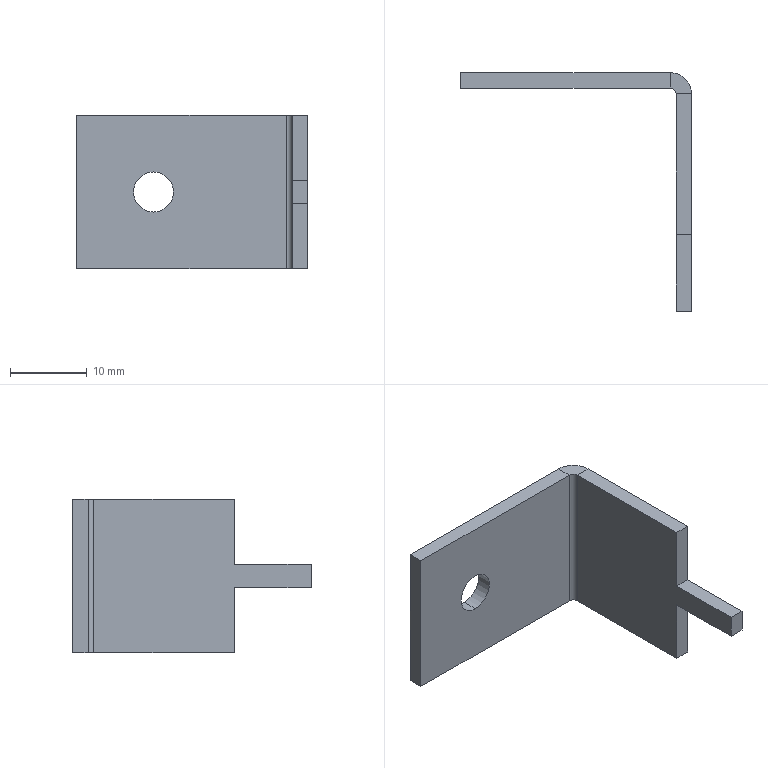Part | SolidWorks | features EdgeFlange 1, FlatPattern 1, HoleWzd 1, ICE 1, SMBaseFlange 1, SheetMetal 1 | 1 solid | 20 faces | box 30 x 31 x 20 mm | volume 1948 mm3 | plane 16 | cylinder 4 | commonest cylinder face diameters 5.2 x2 1.473 x1 5.473 x1
STEP:
#1=CARTESIAN_POINT('',(-5.,0.,2.6));
#2=VERTEX_POINT('',#1);
#3=CARTESIAN_POINT('',(-5.,0.,-2.6));
#4=VERTEX_POINT('',#3);
#5=CARTESIAN_POINT('',(-5.,0.,0.));
#6=DIRECTION('',(0.,-1.,0.));
#7=DIRECTION('',(0.,0.,-1.));
#8=AXIS2_PLACEMENT_3D('',#5,#6,#7);
#9=CIRCLE('',#8,2.6);
#10=EDGE_CURVE('',#2,#4,#9,.T.);
#11=ORIENTED_EDGE('',*,*,#10,.F.);
#12=CARTESIAN_POINT('',(-5.,-2.,2.6));
#13=VERTEX_POINT('',#12);
#14=CARTESIAN_POINT('',(-5.,-2.,2.6));
#15=DIRECTION('',(0.,-1.,0.));
#16=VECTOR('',#15,1000.);
#17=LINE('',#14,#16);
#18=EDGE_CURVE('',#2,#13,#17,.T.);
#19=ORIENTED_EDGE('',*,*,#18,.T.);
#20=CARTESIAN_POINT('',(-5.,-2.,-2.6));
#21=VERTEX_POINT('',#20);
#22=CARTESIAN_POINT('',(-5.,-2.,0.));
#23=DIRECTION('',(0.,-1.,0.));
#24=DIRECTION('',(0.,0.,-1.));
#25=AXIS2_PLACEMENT_3D('',#22,#23,#24);
#26=CIRCLE('',#25,2.6);
#27=EDGE_CURVE('',#13,#21,#26,.T.);
#28=ORIENTED_EDGE('',*,*,#27,.T.);
#29=CARTESIAN_POINT('',(-5.,-2.,-2.6));
#30=DIRECTION('',(0.,-1.,0.));
#31=VECTOR('',#30,1000.);
#32=LINE('',#29,#31);
#33=EDGE_CURVE('',#4,#21,#32,.T.);
#34=ORIENTED_EDGE('',*,*,#33,.F.);
#35=EDGE_LOOP('',(#11,#19,#28,#34));
#36=FACE_OUTER_BOUND('',#35,.T.);
#37=CARTESIAN_POINT('',(-5.,-2.,0.));
#38=DIRECTION('',(0.,-1.,0.));
#39=DIRECTION('',(0.,0.,-1.));
#40=AXIS2_PLACEMENT_3D('',#37,#38,#39);
#41=CYLINDRICAL_SURFACE('',#40,2.6);
#42=ADVANCED_FACE('',(#36),#41,.F.);
#43=CARTESIAN_POINT('',(-15.,-2.,10.));
#44=VERTEX_POINT('',#43);
#45=CARTESIAN_POINT('',(12.263,-2.,10.));
#46=VERTEX_POINT('',#45);
#47=CARTESIAN_POINT('',(-15.,-2.,10.));
#48=DIRECTION('',(1.,0.,0.));
#49=VECTOR('',#48,1000.);
#50=LINE('',#47,#49);
#51=EDGE_CURVE('',#44,#46,#50,.T.);
#52=ORIENTED_EDGE('',*,*,#51,.T.);
#53=CARTESIAN_POINT('',(12.263,0.,10.));
#54=VERTEX_POINT('',#53);
#55=CARTESIAN_POINT('',(12.263,-2.,10.));
#56=DIRECTION('',(0.,1.,0.));
#57=VECTOR('',#56,1000.);
#58=LINE('',#55,#57);
#59=EDGE_CURVE('',#46,#54,#58,.T.);
#60=ORIENTED_EDGE('',*,*,#59,.T.);
#61=CARTESIAN_POINT('',(-15.,0.,10.));
#62=VERTEX_POINT('',#61);
#63=CARTESIAN_POINT('',(-15.,0.,10.));
#64=DIRECTION('',(1.,0.,0.));
#65=VECTOR('',#64,1000.);
#66=LINE('',#63,#65);
#67=EDGE_CURVE('',#62,#54,#66,.T.);
#68=ORIENTED_EDGE('',*,*,#67,.F.);
#69=CARTESIAN_POINT('',(-15.,-2.,10.));
#70=DIRECTION('',(0.,1.,0.));
#71=VECTOR('',#70,1000.);
#72=LINE('',#69,#71);
#73=EDGE_CURVE('',#44,#62,#72,.T.);
#74=ORIENTED_EDGE('',*,*,#73,.F.);
#75=EDGE_LOOP('',(#52,#60,#68,#74));
#76=FACE_OUTER_BOUND('',#75,.T.);
#77=CARTESIAN_POINT('',(-15.,-2.,10.));
#78=DIRECTION('',(0.,0.,1.));
#79=DIRECTION('',(1.,0.,0.));
#80=AXIS2_PLACEMENT_3D('',#77,#78,#79);
#81=PLANE('',#80);
#82=ADVANCED_FACE('',(#76),#81,.T.);
#83=CARTESIAN_POINT('',(-5.,-2.,0.));
#84=DIRECTION('',(0.,-1.,0.));
#85=DIRECTION('',(0.,0.,-1.));
#86=AXIS2_PLACEMENT_3D('',#83,#84,#85);
#87=CIRCLE('',#86,2.6);
#88=EDGE_CURVE('',#21,#13,#87,.T.);
#89=ORIENTED_EDGE('',*,*,#88,.F.);
#90=ORIENTED_EDGE('',*,*,#27,.F.);
#91=EDGE_LOOP('',(#89,#90));
#92=FACE_BOUND('',#91,.T.);
#93=CARTESIAN_POINT('',(12.263,-2.,-10.));
#94=VERTEX_POINT('',#93);
#95=CARTESIAN_POINT('',(12.263,-2.,10.));
#96=DIRECTION('',(0.,0.,-1.));
#97=VECTOR('',#96,1000.);
#98=LINE('',#95,#97);
#99=EDGE_CURVE('',#46,#94,#98,.T.);
#100=ORIENTED_EDGE('',*,*,#99,.F.);
#101=ORIENTED_EDGE('',*,*,#51,.F.);
#102=CARTESIAN_POINT('',(-15.,-2.,-10.));
#103=VERTEX_POINT('',#102);
#104=CARTESIAN_POINT('',(-15.,-2.,-10.));
#105=DIRECTION('',(0.,0.,1.));
#106=VECTOR('',#105,1000.);
#107=LINE('',#104,#106);
#108=EDGE_CURVE('',#103,#44,#107,.T.);
#109=ORIENTED_EDGE('',*,*,#108,.F.);
#110=CARTESIAN_POINT('',(-15.,-2.,-10.));
#111=DIRECTION('',(-1.,0.,0.));
#112=VECTOR('',#111,1000.);
#113=LINE('',#110,#112);
#114=EDGE_CURVE('',#94,#103,#113,.T.);
#115=ORIENTED_EDGE('',*,*,#114,.F.);
#116=EDGE_LOOP('',(#100,#101,#109,#115));
#117=FACE_OUTER_BOUND('',#116,.T.);
#118=CARTESIAN_POINT('',(0.,-2.,0.));
#119=DIRECTION('',(0.,1.,0.));
#120=DIRECTION('',(0.,0.,1.));
#121=AXIS2_PLACEMENT_3D('',#118,#119,#120);
#122=PLANE('',#121);
#123=ADVANCED_FACE('',(#92,#117),#122,.F.);
#124=CARTESIAN_POINT('',(-5.,0.,0.));
#125=DIRECTION('',(0.,-1.,0.));
#126=DIRECTION('',(0.,0.,-1.));
#127=AXIS2_PLACEMENT_3D('',#124,#125,#126);
#128=CIRCLE('',#127,2.6);
#129=EDGE_CURVE('',#4,#2,#128,.T.);
#130=ORIENTED_EDGE('',*,*,#129,.T.);
#131=ORIENTED_EDGE('',*,*,#10,.T.);
#132=EDGE_LOOP('',(#130,#131));
#133=FACE_BOUND('',#132,.T.);
#134=ORIENTED_EDGE('',*,*,#67,.T.);
#135=CARTESIAN_POINT('',(12.263,0.,-10.));
#136=VERTEX_POINT('',#135);
#137=CARTESIAN_POINT('',(12.263,0.,10.));
#138=DIRECTION('',(0.,0.,-1.));
#139=VECTOR('',#138,1000.);
#140=LINE('',#137,#139);
#141=EDGE_CURVE('',#54,#136,#140,.T.);
#142=ORIENTED_EDGE('',*,*,#141,.T.);
#143=CARTESIAN_POINT('',(-15.,0.,-10.));
#144=VERTEX_POINT('',#143);
#145=CARTESIAN_POINT('',(-15.,0.,-10.));
#146=DIRECTION('',(-1.,0.,0.));
#147=VECTOR('',#146,1000.);
#148=LINE('',#145,#147);
#149=EDGE_CURVE('',#136,#144,#148,.T.);
#150=ORIENTED_EDGE('',*,*,#149,.T.);
#151=CARTESIAN_POINT('',(-15.,0.,-10.));
#152=DIRECTION('',(0.,0.,1.));
#153=VECTOR('',#152,1000.);
#154=LINE('',#151,#153);
#155=EDGE_CURVE('',#144,#62,#154,.T.);
#156=ORIENTED_EDGE('',*,*,#155,.T.);
#157=EDGE_LOOP('',(#134,#142,#150,#156));
#158=FACE_OUTER_BOUND('',#157,.T.);
#159=CARTESIAN_POINT('',(0.,0.,0.));
#160=DIRECTION('',(0.,1.,0.));
#161=DIRECTION('',(0.,0.,1.));
#162=AXIS2_PLACEMENT_3D('',#159,#160,#161);
#163=PLANE('',#162);
#164=ADVANCED_FACE('',(#133,#158),#163,.T.);
#165=ORIENTED_EDGE('',*,*,#155,.F.);
#166=CARTESIAN_POINT('',(-15.,-2.,-10.));
#167=DIRECTION('',(0.,1.,0.));
#168=VECTOR('',#167,1000.);
#169=LINE('',#166,#168);
#170=EDGE_CURVE('',#103,#144,#169,.T.);
#171=ORIENTED_EDGE('',*,*,#170,.F.);
#172=ORIENTED_EDGE('',*,*,#108,.T.);
#173=ORIENTED_EDGE('',*,*,#73,.T.);
#174=EDGE_LOOP('',(#165,#171,#172,#173));
#175=FACE_OUTER_BOUND('',#174,.T.);
#176=CARTESIAN_POINT('',(-15.,-2.,-10.));
#177=DIRECTION('',(-1.,0.,0.));
#178=DIRECTION('',(0.,0.,1.));
#179=AXIS2_PLACEMENT_3D('',#176,#177,#178);
#180=PLANE('',#179);
#181=ADVANCED_FACE('',(#175),#180,.T.);
#182=CARTESIAN_POINT('',(12.263,-2.,-10.));
#183=DIRECTION('',(0.,1.,0.));
#184=VECTOR('',#183,1000.);
#185=LINE('',#182,#184);
#186=EDGE_CURVE('',#94,#136,#185,.T.);
#187=ORIENTED_EDGE('',*,*,#186,.F.);
#188=ORIENTED_EDGE('',*,*,#114,.T.);
#189=ORIENTED_EDGE('',*,*,#170,.T.);
#190=ORIENTED_EDGE('',*,*,#149,.F.);
#191=EDGE_LOOP('',(#187,#188,#189,#190));
#192=FACE_OUTER_BOUND('',#191,.T.);
#193=CARTESIAN_POINT('',(-15.,-2.,-10.));
#194=DIRECTION('',(0.,0.,-1.));
#195=DIRECTION('',(-1.,0.,0.));
#196=AXIS2_PLACEMENT_3D('',#193,#194,#195);
#197=PLANE('',#196);
#198=ADVANCED_FACE('',(#192),#197,.T.);
#199=CARTESIAN_POINT('',(13.,-2.737,-10.));
#200=VERTEX_POINT('',#199);
#201=CARTESIAN_POINT('',(15.,-2.737,-10.));
#202=VERTEX_POINT('',#201);
#203=CARTESIAN_POINT('',(15.,-2.737,-10.));
#204=DIRECTION('',(1.,0.,0.));
#205=VECTOR('',#204,1000.);
#206=LINE('',#203,#205);
#207=EDGE_CURVE('',#200,#202,#206,.T.);
#208=ORIENTED_EDGE('',*,*,#207,.F.);
#209=CARTESIAN_POINT('',(12.263,-2.737,-10.));
#210=DIRECTION('',(0.,0.,-1.));
#211=DIRECTION('',(1.,0.,0.));
#212=AXIS2_PLACEMENT_3D('',#209,#210,#211);
#213=CIRCLE('',#212,0.7366);
#214=EDGE_CURVE('',#94,#200,#213,.T.);
#215=ORIENTED_EDGE('',*,*,#214,.F.);
#216=ORIENTED_EDGE('',*,*,#186,.T.);
#217=CARTESIAN_POINT('',(12.263,-2.737,-10.));
#218=DIRECTION('',(0.,0.,-1.));
#219=DIRECTION('',(1.,0.,0.));
#220=AXIS2_PLACEMENT_3D('',#217,#218,#219);
#221=CIRCLE('',#220,2.737);
#222=EDGE_CURVE('',#136,#202,#221,.T.);
#223=ORIENTED_EDGE('',*,*,#222,.T.);
#224=EDGE_LOOP('',(#208,#215,#216,#223));
#225=FACE_OUTER_BOUND('',#224,.T.);
#226=CARTESIAN_POINT('',(12.263,-2.737,-10.));
#227=DIRECTION('',(0.,0.,-1.));
#228=DIRECTION('',(-1.,0.,0.));
#229=AXIS2_PLACEMENT_3D('',#226,#227,#228);
#230=PLANE('',#229);
#231=ADVANCED_FACE('',(#225),#230,.T.);
#232=CARTESIAN_POINT('',(13.,-2.737,10.));
#233=VERTEX_POINT('',#232);
#234=CARTESIAN_POINT('',(12.263,-2.737,10.));
#235=DIRECTION('',(0.,0.,1.));
#236=DIRECTION('',(1.,0.,0.));
#237=AXIS2_PLACEMENT_3D('',#234,#235,#236);
#238=CIRCLE('',#237,0.7366);
#239=EDGE_CURVE('',#233,#46,#238,.T.);
#240=ORIENTED_EDGE('',*,*,#239,.F.);
#241=CARTESIAN_POINT('',(15.,-2.737,10.));
#242=VERTEX_POINT('',#241);
#243=CARTESIAN_POINT('',(13.,-2.737,10.));
#244=DIRECTION('',(1.,0.,0.));
#245=VECTOR('',#244,1000.);
#246=LINE('',#243,#245);
#247=EDGE_CURVE('',#233,#242,#246,.T.);
#248=ORIENTED_EDGE('',*,*,#247,.T.);
#249=CARTESIAN_POINT('',(12.263,-2.737,10.));
#250=DIRECTION('',(0.,0.,1.));
#251=DIRECTION('',(1.,0.,0.));
#252=AXIS2_PLACEMENT_3D('',#249,#250,#251);
#253=CIRCLE('',#252,2.737);
#254=EDGE_CURVE('',#242,#54,#253,.T.);
#255=ORIENTED_EDGE('',*,*,#254,.T.);
#256=ORIENTED_EDGE('',*,*,#59,.F.);
#257=EDGE_LOOP('',(#240,#248,#255,#256));
#258=FACE_OUTER_BOUND('',#257,.T.);
#259=CARTESIAN_POINT('',(12.263,-2.737,10.));
#260=DIRECTION('',(0.,0.,-1.));
#261=DIRECTION('',(-1.,0.,0.));
#262=AXIS2_PLACEMENT_3D('',#259,#260,#261);
#263=PLANE('',#262);
#264=ADVANCED_FACE('',(#258),#263,.F.);
#265=ORIENTED_EDGE('',*,*,#141,.F.);
#266=ORIENTED_EDGE('',*,*,#254,.F.);
#267=CARTESIAN_POINT('',(15.,-2.737,-10.));
#268=DIRECTION('',(0.,0.,-1.));
#269=VECTOR('',#268,1000.);
#270=LINE('',#267,#269);
#271=EDGE_CURVE('',#242,#202,#270,.T.);
#272=ORIENTED_EDGE('',*,*,#271,.T.);
#273=ORIENTED_EDGE('',*,*,#222,.F.);
#274=EDGE_LOOP('',(#265,#266,#272,#273));
#275=FACE_OUTER_BOUND('',#274,.T.);
#276=CARTESIAN_POINT('',(12.263,-2.737,10.));
#277=DIRECTION('',(0.,0.,1.));
#278=DIRECTION('',(1.,0.,0.));
#279=AXIS2_PLACEMENT_3D('',#276,#277,#278);
#280=CYLINDRICAL_SURFACE('',#279,2.737);
#281=ADVANCED_FACE('',(#275),#280,.T.);
#282=ORIENTED_EDGE('',*,*,#99,.T.);
#283=ORIENTED_EDGE('',*,*,#214,.T.);
#284=CARTESIAN_POINT('',(13.,-2.737,-10.));
#285=DIRECTION('',(0.,0.,1.));
#286=VECTOR('',#285,1000.);
#287=LINE('',#284,#286);
#288=EDGE_CURVE('',#200,#233,#287,.T.);
#289=ORIENTED_EDGE('',*,*,#288,.T.);
#290=ORIENTED_EDGE('',*,*,#239,.T.);
#291=EDGE_LOOP('',(#282,#283,#289,#290));
#292=FACE_OUTER_BOUND('',#291,.T.);
#293=CARTESIAN_POINT('',(12.263,-2.737,10.));
#294=DIRECTION('',(0.,0.,1.));
#295=DIRECTION('',(1.,0.,0.));
#296=AXIS2_PLACEMENT_3D('',#293,#294,#295);
#297=CYLINDRICAL_SURFACE('',#296,0.7366);
#298=ADVANCED_FACE('',(#292),#297,.F.);
#299=CARTESIAN_POINT('',(13.,-21.,10.));
#300=VERTEX_POINT('',#299);
#301=CARTESIAN_POINT('',(13.,-31.,10.));
#302=DIRECTION('',(0.,-1.,0.));
#303=VECTOR('',#302,1000.);
#304=LINE('',#301,#303);
#305=EDGE_CURVE('',#233,#300,#304,.T.);
#306=ORIENTED_EDGE('',*,*,#305,.T.);
#307=CARTESIAN_POINT('',(15.,-21.,10.));
#308=VERTEX_POINT('',#307);
#309=CARTESIAN_POINT('',(15.,-21.,10.));
#310=DIRECTION('',(1.,0.,0.));
#311=VECTOR('',#310,1000.);
#312=LINE('',#309,#311);
#313=EDGE_CURVE('',#300,#308,#312,.T.);
#314=ORIENTED_EDGE('',*,*,#313,.T.);
#315=CARTESIAN_POINT('',(15.,0.,10.));
#316=DIRECTION('',(0.,-1.,0.));
#317=VECTOR('',#316,1000.);
#318=LINE('',#315,#317);
#319=EDGE_CURVE('',#242,#308,#318,.T.);
#320=ORIENTED_EDGE('',*,*,#319,.F.);
#321=ORIENTED_EDGE('',*,*,#247,.F.);
#322=EDGE_LOOP('',(#306,#314,#320,#321));
#323=FACE_OUTER_BOUND('',#322,.T.);
#324=CARTESIAN_POINT('',(15.,-31.,10.));
#325=DIRECTION('',(0.,0.,-1.));
#326=DIRECTION('',(-1.,0.,0.));
#327=AXIS2_PLACEMENT_3D('',#324,#325,#326);
#328=PLANE('',#327);
#329=ADVANCED_FACE('',(#323),#328,.F.);
#330=CARTESIAN_POINT('',(15.,-21.,-10.));
#331=VERTEX_POINT('',#330);
#332=CARTESIAN_POINT('',(15.,0.,-10.));
#333=DIRECTION('',(0.,1.,0.));
#334=VECTOR('',#333,1000.);
#335=LINE('',#332,#334);
#336=EDGE_CURVE('',#331,#202,#335,.T.);
#337=ORIENTED_EDGE('',*,*,#336,.F.);
#338=CARTESIAN_POINT('',(13.,-21.,-10.));
#339=VERTEX_POINT('',#338);
#340=CARTESIAN_POINT('',(15.,-21.,-10.));
#341=DIRECTION('',(-1.,0.,0.));
#342=VECTOR('',#341,1000.);
#343=LINE('',#340,#342);
#344=EDGE_CURVE('',#331,#339,#343,.T.);
#345=ORIENTED_EDGE('',*,*,#344,.T.);
#346=CARTESIAN_POINT('',(13.,-2.,-10.));
#347=DIRECTION('',(0.,1.,0.));
#348=VECTOR('',#347,1000.);
#349=LINE('',#346,#348);
#350=EDGE_CURVE('',#339,#200,#349,.T.);
#351=ORIENTED_EDGE('',*,*,#350,.T.);
#352=ORIENTED_EDGE('',*,*,#207,.T.);
#353=EDGE_LOOP('',(#337,#345,#351,#352));
#354=FACE_OUTER_BOUND('',#353,.T.);
#355=CARTESIAN_POINT('',(15.,-2.,-10.));
#356=DIRECTION('',(0.,0.,1.));
#357=DIRECTION('',(1.,0.,0.));
#358=AXIS2_PLACEMENT_3D('',#355,#356,#357);
#359=PLANE('',#358);
#360=ADVANCED_FACE('',(#354),#359,.F.);
#361=ORIENTED_EDGE('',*,*,#319,.T.);
#362=CARTESIAN_POINT('',(15.,-21.,1.5));
#363=VERTEX_POINT('',#362);
#364=CARTESIAN_POINT('',(15.,-21.,17.733));
#365=DIRECTION('',(0.,0.,1.));
#366=VECTOR('',#365,1000.);
#367=LINE('',#364,#366);
#368=EDGE_CURVE('',#363,#308,#367,.T.);
#369=ORIENTED_EDGE('',*,*,#368,.F.);
#370=CARTESIAN_POINT('',(15.,-31.,1.5));
#371=VERTEX_POINT('',#370);
#372=CARTESIAN_POINT('',(15.,-21.,1.5));
#373=DIRECTION('',(0.,1.,0.));
#374=VECTOR('',#373,1000.);
#375=LINE('',#372,#374);
#376=EDGE_CURVE('',#371,#363,#375,.T.);
#377=ORIENTED_EDGE('',*,*,#376,.F.);
#378=CARTESIAN_POINT('',(15.,-31.,-1.5));
#379=VERTEX_POINT('',#378);
#380=CARTESIAN_POINT('',(15.,-31.,0.));
#381=DIRECTION('',(0.,0.,-1.));
#382=VECTOR('',#381,1000.);
#383=LINE('',#380,#382);
#384=EDGE_CURVE('',#371,#379,#383,.T.);
#385=ORIENTED_EDGE('',*,*,#384,.T.);
#386=CARTESIAN_POINT('',(15.,-21.,-1.5));
#387=VERTEX_POINT('',#386);
#388=CARTESIAN_POINT('',(15.,-31.,-1.5));
#389=DIRECTION('',(0.,-1.,0.));
#390=VECTOR('',#389,1000.);
#391=LINE('',#388,#390);
#392=EDGE_CURVE('',#387,#379,#391,.T.);
#393=ORIENTED_EDGE('',*,*,#392,.F.);
#394=CARTESIAN_POINT('',(15.,-21.,-1.5));
#395=DIRECTION('',(0.,0.,1.));
#396=VECTOR('',#395,1000.);
#397=LINE('',#394,#396);
#398=EDGE_CURVE('',#331,#387,#397,.T.);
#399=ORIENTED_EDGE('',*,*,#398,.F.);
#400=ORIENTED_EDGE('',*,*,#336,.T.);
#401=ORIENTED_EDGE('',*,*,#271,.F.);
#402=EDGE_LOOP('',(#361,#369,#377,#385,#393,#399,#400,#401));
#403=FACE_OUTER_BOUND('',#402,.T.);
#404=CARTESIAN_POINT('',(15.,0.,0.));
#405=DIRECTION('',(-1.,0.,0.));
#406=DIRECTION('',(0.,-1.,0.));
#407=AXIS2_PLACEMENT_3D('',#404,#405,#406);
#408=PLANE('',#407);
#409=ADVANCED_FACE('',(#403),#408,.F.);
#410=CARTESIAN_POINT('',(13.,-21.,1.5));
#411=VERTEX_POINT('',#410);
#412=CARTESIAN_POINT('',(13.,-21.,0.));
#413=DIRECTION('',(0.,0.,-1.));
#414=VECTOR('',#413,1000.);
#415=LINE('',#412,#414);
#416=EDGE_CURVE('',#300,#411,#415,.T.);
#417=ORIENTED_EDGE('',*,*,#416,.F.);
#418=ORIENTED_EDGE('',*,*,#305,.F.);
#419=ORIENTED_EDGE('',*,*,#288,.F.);
#420=ORIENTED_EDGE('',*,*,#350,.F.);
#421=CARTESIAN_POINT('',(13.,-21.,-1.5));
#422=VERTEX_POINT('',#421);
#423=CARTESIAN_POINT('',(13.,-21.,0.));
#424=DIRECTION('',(0.,0.,-1.));
#425=VECTOR('',#424,1000.);
#426=LINE('',#423,#425);
#427=EDGE_CURVE('',#422,#339,#426,.T.);
#428=ORIENTED_EDGE('',*,*,#427,.F.);
#429=CARTESIAN_POINT('',(13.,-31.,-1.5));
#430=VERTEX_POINT('',#429);
#431=CARTESIAN_POINT('',(13.,0.,-1.5));
#432=DIRECTION('',(0.,1.,0.));
#433=VECTOR('',#432,1000.);
#434=LINE('',#431,#433);
#435=EDGE_CURVE('',#430,#422,#434,.T.);
#436=ORIENTED_EDGE('',*,*,#435,.F.);
#437=CARTESIAN_POINT('',(13.,-31.,1.5));
#438=VERTEX_POINT('',#437);
#439=CARTESIAN_POINT('',(13.,-31.,-10.));
#440=DIRECTION('',(0.,0.,-1.));
#441=VECTOR('',#440,1000.);
#442=LINE('',#439,#441);
#443=EDGE_CURVE('',#438,#430,#442,.T.);
#444=ORIENTED_EDGE('',*,*,#443,.F.);
#445=CARTESIAN_POINT('',(13.,0.,1.5));
#446=DIRECTION('',(0.,-1.,0.));
#447=VECTOR('',#446,1000.);
#448=LINE('',#445,#447);
#449=EDGE_CURVE('',#411,#438,#448,.T.);
#450=ORIENTED_EDGE('',*,*,#449,.F.);
#451=EDGE_LOOP('',(#417,#418,#419,#420,#428,#436,#444,#450));
#452=FACE_OUTER_BOUND('',#451,.T.);
#453=CARTESIAN_POINT('',(13.,0.,0.));
#454=DIRECTION('',(-1.,0.,0.));
#455=DIRECTION('',(0.,-1.,0.));
#456=AXIS2_PLACEMENT_3D('',#453,#454,#455);
#457=PLANE('',#456);
#458=ADVANCED_FACE('',(#452),#457,.T.);
#459=ORIENTED_EDGE('',*,*,#384,.F.);
#460=CARTESIAN_POINT('',(15.,-31.,1.5));
#461=DIRECTION('',(-1.,0.,0.));
#462=VECTOR('',#461,1000.);
#463=LINE('',#460,#462);
#464=EDGE_CURVE('',#371,#438,#463,.T.);
#465=ORIENTED_EDGE('',*,*,#464,.T.);
#466=ORIENTED_EDGE('',*,*,#443,.T.);
#467=CARTESIAN_POINT('',(15.,-31.,-1.5));
#468=DIRECTION('',(1.,0.,0.));
#469=VECTOR('',#468,1000.);
#470=LINE('',#467,#469);
#471=EDGE_CURVE('',#430,#379,#470,.T.);
#472=ORIENTED_EDGE('',*,*,#471,.T.);
#473=EDGE_LOOP('',(#459,#465,#466,#472));
#474=FACE_OUTER_BOUND('',#473,.T.);
#475=CARTESIAN_POINT('',(15.,-31.,-10.));
#476=DIRECTION('',(0.,1.,0.));
#477=DIRECTION('',(-1.,0.,0.));
#478=AXIS2_PLACEMENT_3D('',#475,#476,#477);
#479=PLANE('',#478);
#480=ADVANCED_FACE('',(#474),#479,.F.);
#481=ORIENTED_EDGE('',*,*,#435,.T.);
#482=CARTESIAN_POINT('',(-15.,-21.,-1.5));
#483=DIRECTION('',(1.,0.,0.));
#484=VECTOR('',#483,1000.);
#485=LINE('',#482,#484);
#486=EDGE_CURVE('',#422,#387,#485,.T.);
#487=ORIENTED_EDGE('',*,*,#486,.T.);
#488=ORIENTED_EDGE('',*,*,#392,.T.);
#489=ORIENTED_EDGE('',*,*,#471,.F.);
#490=EDGE_LOOP('',(#481,#487,#488,#489));
#491=FACE_OUTER_BOUND('',#490,.T.);
#492=CARTESIAN_POINT('',(-15.,-31.,-1.5));
#493=DIRECTION('',(0.,0.,1.));
#494=DIRECTION('',(0.,-1.,0.));
#495=AXIS2_PLACEMENT_3D('',#492,#493,#494);
#496=PLANE('',#495);
#497=ADVANCED_FACE('',(#491),#496,.F.);
#498=ORIENTED_EDGE('',*,*,#398,.T.);
#499=ORIENTED_EDGE('',*,*,#486,.F.);
#500=ORIENTED_EDGE('',*,*,#427,.T.);
#501=ORIENTED_EDGE('',*,*,#344,.F.);
#502=EDGE_LOOP('',(#498,#499,#500,#501));
#503=FACE_OUTER_BOUND('',#502,.T.);
#504=CARTESIAN_POINT('',(-15.,-21.,-1.5));
#505=DIRECTION('',(0.,1.,0.));
#506=DIRECTION('',(-1.,0.,0.));
#507=AXIS2_PLACEMENT_3D('',#504,#505,#506);
#508=PLANE('',#507);
#509=ADVANCED_FACE('',(#503),#508,.F.);
#510=ORIENTED_EDGE('',*,*,#416,.T.);
#511=CARTESIAN_POINT('',(-15.,-21.,1.5));
#512=DIRECTION('',(1.,0.,0.));
#513=VECTOR('',#512,1000.);
#514=LINE('',#511,#513);
#515=EDGE_CURVE('',#411,#363,#514,.T.);
#516=ORIENTED_EDGE('',*,*,#515,.T.);
#517=ORIENTED_EDGE('',*,*,#368,.T.);
#518=ORIENTED_EDGE('',*,*,#313,.F.);
#519=EDGE_LOOP('',(#510,#516,#517,#518));
#520=FACE_OUTER_BOUND('',#519,.T.);
#521=CARTESIAN_POINT('',(-15.,-21.,17.733));
#522=DIRECTION('',(0.,1.,0.));
#523=DIRECTION('',(-1.,0.,0.));
#524=AXIS2_PLACEMENT_3D('',#521,#522,#523);
#525=PLANE('',#524);
#526=ADVANCED_FACE('',(#520),#525,.F.);
#527=ORIENTED_EDGE('',*,*,#449,.T.);
#528=ORIENTED_EDGE('',*,*,#464,.F.);
#529=ORIENTED_EDGE('',*,*,#376,.T.);
#530=ORIENTED_EDGE('',*,*,#515,.F.);
#531=EDGE_LOOP('',(#527,#528,#529,#530));
#532=FACE_OUTER_BOUND('',#531,.T.);
#533=CARTESIAN_POINT('',(-15.,-21.,1.5));
#534=DIRECTION('',(0.,0.,-1.));
#535=DIRECTION('',(0.,1.,0.));
#536=AXIS2_PLACEMENT_3D('',#533,#534,#535);
#537=PLANE('',#536);
#538=ADVANCED_FACE('',(#532),#537,.F.);
#539=ORIENTED_EDGE('',*,*,#18,.F.);
#540=ORIENTED_EDGE('',*,*,#129,.F.);
#541=ORIENTED_EDGE('',*,*,#33,.T.);
#542=ORIENTED_EDGE('',*,*,#88,.T.);
#543=EDGE_LOOP('',(#539,#540,#541,#542));
#544=FACE_OUTER_BOUND('',#543,.T.);
#545=CARTESIAN_POINT('',(-5.,-2.,0.));
#546=DIRECTION('',(0.,-1.,0.));
#547=DIRECTION('',(0.,0.,-1.));
#548=AXIS2_PLACEMENT_3D('',#545,#546,#547);
#549=CYLINDRICAL_SURFACE('',#548,2.6);
#550=ADVANCED_FACE('',(#544),#549,.F.);
#551=CLOSED_SHELL('',(#42,#82,#123,#164,#181,#198,#231,#264,#281,#298,#329,#360,#409,#458,#480,#497,#509,#526,#538,#550));
#552=MANIFOLD_SOLID_BREP('',#551);
#553=CARTESIAN_POINT('',(0.,0.,0.));
#554=DIRECTION('',(0.,0.,1.));
#555=DIRECTION('',(1.,0.,0.));
#556=AXIS2_PLACEMENT_3D('',#553,#554,#555);
#557=(LENGTH_UNIT()NAMED_UNIT(*)SI_UNIT(.MILLI.,.METRE.));
#558=UNCERTAINTY_MEASURE_WITH_UNIT(LENGTH_MEASURE(0.00001),#557,'','');
#559=(NAMED_UNIT(*)PLANE_ANGLE_UNIT()SI_UNIT($,.RADIAN.));
#560=(NAMED_UNIT(*)SI_UNIT($,.STERADIAN.)SOLID_ANGLE_UNIT());
#561=(GEOMETRIC_REPRESENTATION_CONTEXT(3)GLOBAL_UNCERTAINTY_ASSIGNED_CONTEXT((#558))GLOBAL_UNIT_ASSIGNED_CONTEXT((#557,#559,#560))REPRESENTATION_CONTEXT('',''));
#562=ADVANCED_BREP_SHAPE_REPRESENTATION('',(#552,#556),#561);